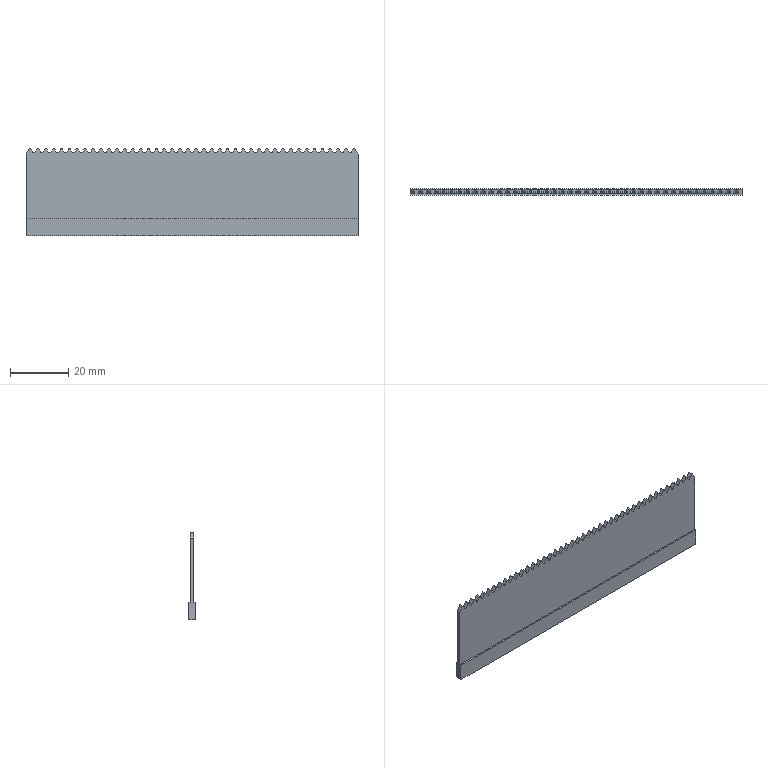Part | STEP file | 1 solid | 176 faces | box 114.24 x 2.3 x 30 mm | volume 5016 mm3 | plane 93 | cylinder 83 | commonest cylinder face diameters 0.5 x42 0.8 x41